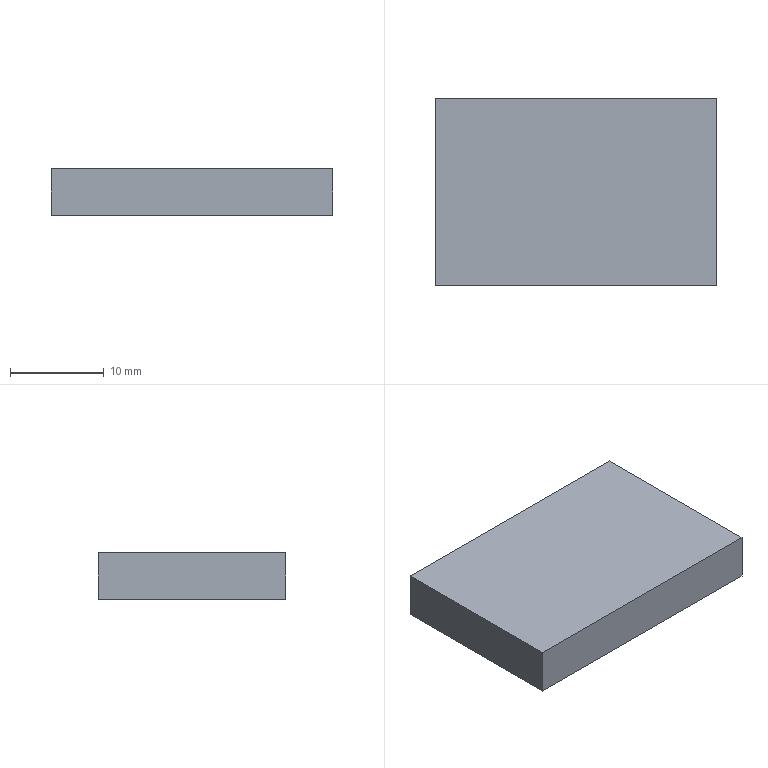Part | STEP file | MISUMI magnet MGLF5-30-20 | 1 solid | 6 faces | box 30 x 20 x 5 mm | volume 3000 mm3 | plane 6
STEP:
#1=CARTESIAN_POINT('',(0.,0.,0.));
#2=DIRECTION('',(0.,0.,1.));
#3=DIRECTION('',(1.,0.,0.));
#4=AXIS2_PLACEMENT_3D('',#1,#2,#3);
#5=CARTESIAN_POINT('',(15.,-10.,5.));
#6=VERTEX_POINT('',#5);
#7=CARTESIAN_POINT('',(15.,10.,5.));
#8=VERTEX_POINT('',#7);
#9=CARTESIAN_POINT('',(15.,0.,5.));
#10=DIRECTION('',(0.,1.,0.));
#11=VECTOR('',#10,1.);
#12=LINE('',#9,#11);
#13=CARTESIAN_POINT('',(0.,0.,5.));
#14=DIRECTION('',(0.,0.,1.));
#15=DIRECTION('',(1.,0.,0.));
#16=AXIS2_PLACEMENT_3D('',#13,#14,#15);
#17=PLANE('',#16);
#18=CARTESIAN_POINT('',(15.,0.));
#19=DIRECTION('',(0.,1.));
#20=VECTOR('',#19,1.);
#21=LINE('',#18,#20);
#22=(GEOMETRIC_REPRESENTATION_CONTEXT(2)PARAMETRIC_REPRESENTATION_CONTEXT()REPRESENTATION_CONTEXT('',''));
#23=DEFINITIONAL_REPRESENTATION('',(#21),#22);
#24=PCURVE('',#17,#23);
#25=CARTESIAN_POINT('',(15.,10.,0.));
#26=DIRECTION('',(1.,0.,0.));
#27=DIRECTION('',(0.,0.,-1.));
#28=AXIS2_PLACEMENT_3D('',#25,#26,#27);
#29=PLANE('',#28);
#30=CARTESIAN_POINT('',(-5.,-10.));
#31=DIRECTION('',(0.,1.));
#32=VECTOR('',#31,1.);
#33=LINE('',#30,#32);
#34=(GEOMETRIC_REPRESENTATION_CONTEXT(2)PARAMETRIC_REPRESENTATION_CONTEXT()REPRESENTATION_CONTEXT('',''));
#35=DEFINITIONAL_REPRESENTATION('',(#33),#34);
#36=PCURVE('',#29,#35);
#37=SURFACE_CURVE('',#12,(#24,#36),.PCURVE_S1.);
#38=EDGE_CURVE('',#6,#8,#37,.T.);
#39=ORIENTED_EDGE('',*,*,#38,.T.);
#40=CARTESIAN_POINT('',(-15.,10.,5.));
#41=VERTEX_POINT('',#40);
#42=CARTESIAN_POINT('',(0.,10.,5.));
#43=DIRECTION('',(-1.,0.,0.));
#44=VECTOR('',#43,1.);
#45=LINE('',#42,#44);
#46=CARTESIAN_POINT('',(0.,10.));
#47=DIRECTION('',(-1.,0.));
#48=VECTOR('',#47,1.);
#49=LINE('',#46,#48);
#50=(GEOMETRIC_REPRESENTATION_CONTEXT(2)PARAMETRIC_REPRESENTATION_CONTEXT()REPRESENTATION_CONTEXT('',''));
#51=DEFINITIONAL_REPRESENTATION('',(#49),#50);
#52=PCURVE('',#17,#51);
#53=CARTESIAN_POINT('',(-15.,10.,0.));
#54=DIRECTION('',(0.,1.,0.));
#55=DIRECTION('',(0.,0.,1.));
#56=AXIS2_PLACEMENT_3D('',#53,#54,#55);
#57=PLANE('',#56);
#58=CARTESIAN_POINT('',(5.,15.));
#59=DIRECTION('',(0.,-1.));
#60=VECTOR('',#59,1.);
#61=LINE('',#58,#60);
#62=(GEOMETRIC_REPRESENTATION_CONTEXT(2)PARAMETRIC_REPRESENTATION_CONTEXT()REPRESENTATION_CONTEXT('',''));
#63=DEFINITIONAL_REPRESENTATION('',(#61),#62);
#64=PCURVE('',#57,#63);
#65=SURFACE_CURVE('',#45,(#52,#64),.PCURVE_S1.);
#66=EDGE_CURVE('',#8,#41,#65,.T.);
#67=ORIENTED_EDGE('',*,*,#66,.T.);
#68=CARTESIAN_POINT('',(-15.,-10.,5.));
#69=VERTEX_POINT('',#68);
#70=CARTESIAN_POINT('',(-15.,0.,5.));
#71=DIRECTION('',(0.,-1.,0.));
#72=VECTOR('',#71,1.);
#73=LINE('',#70,#72);
#74=CARTESIAN_POINT('',(-15.,0.));
#75=DIRECTION('',(0.,-1.));
#76=VECTOR('',#75,1.);
#77=LINE('',#74,#76);
#78=(GEOMETRIC_REPRESENTATION_CONTEXT(2)PARAMETRIC_REPRESENTATION_CONTEXT()REPRESENTATION_CONTEXT('',''));
#79=DEFINITIONAL_REPRESENTATION('',(#77),#78);
#80=PCURVE('',#17,#79);
#81=CARTESIAN_POINT('',(-15.,-10.,0.));
#82=DIRECTION('',(-1.,0.,0.));
#83=DIRECTION('',(0.,0.,1.));
#84=AXIS2_PLACEMENT_3D('',#81,#82,#83);
#85=PLANE('',#84);
#86=CARTESIAN_POINT('',(5.,10.));
#87=DIRECTION('',(0.,-1.));
#88=VECTOR('',#87,1.);
#89=LINE('',#86,#88);
#90=(GEOMETRIC_REPRESENTATION_CONTEXT(2)PARAMETRIC_REPRESENTATION_CONTEXT()REPRESENTATION_CONTEXT('',''));
#91=DEFINITIONAL_REPRESENTATION('',(#89),#90);
#92=PCURVE('',#85,#91);
#93=SURFACE_CURVE('',#73,(#80,#92),.PCURVE_S1.);
#94=EDGE_CURVE('',#41,#69,#93,.T.);
#95=ORIENTED_EDGE('',*,*,#94,.T.);
#96=CARTESIAN_POINT('',(0.,-10.,5.));
#97=DIRECTION('',(1.,0.,0.));
#98=VECTOR('',#97,1.);
#99=LINE('',#96,#98);
#100=CARTESIAN_POINT('',(0.,-10.));
#101=DIRECTION('',(1.,0.));
#102=VECTOR('',#101,1.);
#103=LINE('',#100,#102);
#104=(GEOMETRIC_REPRESENTATION_CONTEXT(2)PARAMETRIC_REPRESENTATION_CONTEXT()REPRESENTATION_CONTEXT('',''));
#105=DEFINITIONAL_REPRESENTATION('',(#103),#104);
#106=PCURVE('',#17,#105);
#107=CARTESIAN_POINT('',(15.,-10.,0.));
#108=DIRECTION('',(0.,-1.,0.));
#109=DIRECTION('',(0.,0.,-1.));
#110=AXIS2_PLACEMENT_3D('',#107,#108,#109);
#111=PLANE('',#110);
#112=CARTESIAN_POINT('',(-5.,-15.));
#113=DIRECTION('',(0.,1.));
#114=VECTOR('',#113,1.);
#115=LINE('',#112,#114);
#116=(GEOMETRIC_REPRESENTATION_CONTEXT(2)PARAMETRIC_REPRESENTATION_CONTEXT()REPRESENTATION_CONTEXT('',''));
#117=DEFINITIONAL_REPRESENTATION('',(#115),#116);
#118=PCURVE('',#111,#117);
#119=SURFACE_CURVE('',#99,(#106,#118),.PCURVE_S1.);
#120=EDGE_CURVE('',#69,#6,#119,.T.);
#121=ORIENTED_EDGE('',*,*,#120,.T.);
#122=EDGE_LOOP('',(#39,#67,#95,#121));
#123=FACE_BOUND('',#122,.T.);
#124=ADVANCED_FACE('',(#123),#17,.T.);
#125=CARTESIAN_POINT('',(15.,10.,0.));
#126=VERTEX_POINT('',#125);
#127=CARTESIAN_POINT('',(-15.,10.,0.));
#128=VERTEX_POINT('',#127);
#129=CARTESIAN_POINT('',(-15.,10.,0.));
#130=DIRECTION('',(-1.,0.,0.));
#131=VECTOR('',#130,1.);
#132=LINE('',#129,#131);
#133=CARTESIAN_POINT('',(0.,0.));
#134=DIRECTION('',(0.,-1.));
#135=VECTOR('',#134,1.);
#136=LINE('',#133,#135);
#137=(GEOMETRIC_REPRESENTATION_CONTEXT(2)PARAMETRIC_REPRESENTATION_CONTEXT()REPRESENTATION_CONTEXT('',''));
#138=DEFINITIONAL_REPRESENTATION('',(#136),#137);
#139=PCURVE('',#57,#138);
#140=CARTESIAN_POINT('',(0.,0.,0.));
#141=DIRECTION('',(0.,0.,1.));
#142=DIRECTION('',(1.,0.,0.));
#143=AXIS2_PLACEMENT_3D('',#140,#141,#142);
#144=PLANE('',#143);
#145=CARTESIAN_POINT('',(-15.,10.));
#146=DIRECTION('',(-1.,0.));
#147=VECTOR('',#146,1.);
#148=LINE('',#145,#147);
#149=(GEOMETRIC_REPRESENTATION_CONTEXT(2)PARAMETRIC_REPRESENTATION_CONTEXT()REPRESENTATION_CONTEXT('',''));
#150=DEFINITIONAL_REPRESENTATION('',(#148),#149);
#151=PCURVE('',#144,#150);
#152=SURFACE_CURVE('',#132,(#139,#151),.PCURVE_S1.);
#153=EDGE_CURVE('',#126,#128,#152,.T.);
#154=ORIENTED_EDGE('',*,*,#153,.T.);
#155=CARTESIAN_POINT('',(-15.,10.,0.));
#156=DIRECTION('',(0.,0.,1.));
#157=VECTOR('',#156,1.);
#158=LINE('',#155,#157);
#159=CARTESIAN_POINT('',(0.,0.));
#160=DIRECTION('',(1.,0.));
#161=VECTOR('',#160,1.);
#162=LINE('',#159,#161);
#163=(GEOMETRIC_REPRESENTATION_CONTEXT(2)PARAMETRIC_REPRESENTATION_CONTEXT()REPRESENTATION_CONTEXT('',''));
#164=DEFINITIONAL_REPRESENTATION('',(#162),#163);
#165=PCURVE('',#57,#164);
#166=CARTESIAN_POINT('',(0.,20.));
#167=DIRECTION('',(1.,0.));
#168=VECTOR('',#167,1.);
#169=LINE('',#166,#168);
#170=(GEOMETRIC_REPRESENTATION_CONTEXT(2)PARAMETRIC_REPRESENTATION_CONTEXT()REPRESENTATION_CONTEXT('',''));
#171=DEFINITIONAL_REPRESENTATION('',(#169),#170);
#172=PCURVE('',#85,#171);
#173=SURFACE_CURVE('',#158,(#165,#172),.PCURVE_S1.);
#174=EDGE_CURVE('',#128,#41,#173,.T.);
#175=ORIENTED_EDGE('',*,*,#174,.T.);
#176=ORIENTED_EDGE('',*,*,#66,.F.);
#177=CARTESIAN_POINT('',(15.,10.,0.));
#178=DIRECTION('',(0.,0.,-1.));
#179=VECTOR('',#178,1.);
#180=LINE('',#177,#179);
#181=CARTESIAN_POINT('',(0.,30.));
#182=DIRECTION('',(-1.,0.));
#183=VECTOR('',#182,1.);
#184=LINE('',#181,#183);
#185=(GEOMETRIC_REPRESENTATION_CONTEXT(2)PARAMETRIC_REPRESENTATION_CONTEXT()REPRESENTATION_CONTEXT('',''));
#186=DEFINITIONAL_REPRESENTATION('',(#184),#185);
#187=PCURVE('',#57,#186);
#188=CARTESIAN_POINT('',(0.,0.));
#189=DIRECTION('',(1.,0.));
#190=VECTOR('',#189,1.);
#191=LINE('',#188,#190);
#192=(GEOMETRIC_REPRESENTATION_CONTEXT(2)PARAMETRIC_REPRESENTATION_CONTEXT()REPRESENTATION_CONTEXT('',''));
#193=DEFINITIONAL_REPRESENTATION('',(#191),#192);
#194=PCURVE('',#29,#193);
#195=SURFACE_CURVE('',#180,(#187,#194),.PCURVE_S1.);
#196=EDGE_CURVE('',#8,#126,#195,.T.);
#197=ORIENTED_EDGE('',*,*,#196,.T.);
#198=EDGE_LOOP('',(#154,#175,#176,#197));
#199=FACE_BOUND('',#198,.T.);
#200=ADVANCED_FACE('',(#199),#57,.T.);
#201=CARTESIAN_POINT('',(15.,-10.,0.));
#202=VERTEX_POINT('',#201);
#203=CARTESIAN_POINT('',(15.,10.,0.));
#204=DIRECTION('',(0.,1.,0.));
#205=VECTOR('',#204,1.);
#206=LINE('',#203,#205);
#207=CARTESIAN_POINT('',(0.,0.));
#208=DIRECTION('',(0.,1.));
#209=VECTOR('',#208,1.);
#210=LINE('',#207,#209);
#211=(GEOMETRIC_REPRESENTATION_CONTEXT(2)PARAMETRIC_REPRESENTATION_CONTEXT()REPRESENTATION_CONTEXT('',''));
#212=DEFINITIONAL_REPRESENTATION('',(#210),#211);
#213=PCURVE('',#29,#212);
#214=CARTESIAN_POINT('',(15.,10.));
#215=DIRECTION('',(0.,1.));
#216=VECTOR('',#215,1.);
#217=LINE('',#214,#216);
#218=(GEOMETRIC_REPRESENTATION_CONTEXT(2)PARAMETRIC_REPRESENTATION_CONTEXT()REPRESENTATION_CONTEXT('',''));
#219=DEFINITIONAL_REPRESENTATION('',(#217),#218);
#220=PCURVE('',#144,#219);
#221=SURFACE_CURVE('',#206,(#213,#220),.PCURVE_S1.);
#222=EDGE_CURVE('',#202,#126,#221,.T.);
#223=ORIENTED_EDGE('',*,*,#222,.T.);
#224=ORIENTED_EDGE('',*,*,#196,.F.);
#225=ORIENTED_EDGE('',*,*,#38,.F.);
#226=CARTESIAN_POINT('',(15.,-10.,0.));
#227=DIRECTION('',(0.,0.,-1.));
#228=VECTOR('',#227,1.);
#229=LINE('',#226,#228);
#230=CARTESIAN_POINT('',(0.,-20.));
#231=DIRECTION('',(1.,0.));
#232=VECTOR('',#231,1.);
#233=LINE('',#230,#232);
#234=(GEOMETRIC_REPRESENTATION_CONTEXT(2)PARAMETRIC_REPRESENTATION_CONTEXT()REPRESENTATION_CONTEXT('',''));
#235=DEFINITIONAL_REPRESENTATION('',(#233),#234);
#236=PCURVE('',#29,#235);
#237=CARTESIAN_POINT('',(0.,0.));
#238=DIRECTION('',(1.,0.));
#239=VECTOR('',#238,1.);
#240=LINE('',#237,#239);
#241=(GEOMETRIC_REPRESENTATION_CONTEXT(2)PARAMETRIC_REPRESENTATION_CONTEXT()REPRESENTATION_CONTEXT('',''));
#242=DEFINITIONAL_REPRESENTATION('',(#240),#241);
#243=PCURVE('',#111,#242);
#244=SURFACE_CURVE('',#229,(#236,#243),.PCURVE_S1.);
#245=EDGE_CURVE('',#6,#202,#244,.T.);
#246=ORIENTED_EDGE('',*,*,#245,.T.);
#247=EDGE_LOOP('',(#223,#224,#225,#246));
#248=FACE_BOUND('',#247,.T.);
#249=ADVANCED_FACE('',(#248),#29,.T.);
#250=CARTESIAN_POINT('',(-15.,-10.,0.));
#251=VERTEX_POINT('',#250);
#252=CARTESIAN_POINT('',(15.,-10.,0.));
#253=DIRECTION('',(1.,0.,0.));
#254=VECTOR('',#253,1.);
#255=LINE('',#252,#254);
#256=CARTESIAN_POINT('',(0.,0.));
#257=DIRECTION('',(0.,1.));
#258=VECTOR('',#257,1.);
#259=LINE('',#256,#258);
#260=(GEOMETRIC_REPRESENTATION_CONTEXT(2)PARAMETRIC_REPRESENTATION_CONTEXT()REPRESENTATION_CONTEXT('',''));
#261=DEFINITIONAL_REPRESENTATION('',(#259),#260);
#262=PCURVE('',#111,#261);
#263=CARTESIAN_POINT('',(15.,-10.));
#264=DIRECTION('',(1.,0.));
#265=VECTOR('',#264,1.);
#266=LINE('',#263,#265);
#267=(GEOMETRIC_REPRESENTATION_CONTEXT(2)PARAMETRIC_REPRESENTATION_CONTEXT()REPRESENTATION_CONTEXT('',''));
#268=DEFINITIONAL_REPRESENTATION('',(#266),#267);
#269=PCURVE('',#144,#268);
#270=SURFACE_CURVE('',#255,(#262,#269),.PCURVE_S1.);
#271=EDGE_CURVE('',#251,#202,#270,.T.);
#272=ORIENTED_EDGE('',*,*,#271,.T.);
#273=ORIENTED_EDGE('',*,*,#245,.F.);
#274=ORIENTED_EDGE('',*,*,#120,.F.);
#275=CARTESIAN_POINT('',(-15.,-10.,0.));
#276=DIRECTION('',(0.,0.,-1.));
#277=VECTOR('',#276,1.);
#278=LINE('',#275,#277);
#279=CARTESIAN_POINT('',(0.,-30.));
#280=DIRECTION('',(1.,0.));
#281=VECTOR('',#280,1.);
#282=LINE('',#279,#281);
#283=(GEOMETRIC_REPRESENTATION_CONTEXT(2)PARAMETRIC_REPRESENTATION_CONTEXT()REPRESENTATION_CONTEXT('',''));
#284=DEFINITIONAL_REPRESENTATION('',(#282),#283);
#285=PCURVE('',#111,#284);
#286=CARTESIAN_POINT('',(0.,0.));
#287=DIRECTION('',(-1.,0.));
#288=VECTOR('',#287,1.);
#289=LINE('',#286,#288);
#290=(GEOMETRIC_REPRESENTATION_CONTEXT(2)PARAMETRIC_REPRESENTATION_CONTEXT()REPRESENTATION_CONTEXT('',''));
#291=DEFINITIONAL_REPRESENTATION('',(#289),#290);
#292=PCURVE('',#85,#291);
#293=SURFACE_CURVE('',#278,(#285,#292),.PCURVE_S1.);
#294=EDGE_CURVE('',#69,#251,#293,.T.);
#295=ORIENTED_EDGE('',*,*,#294,.T.);
#296=EDGE_LOOP('',(#272,#273,#274,#295));
#297=FACE_BOUND('',#296,.T.);
#298=ADVANCED_FACE('',(#297),#111,.T.);
#299=CARTESIAN_POINT('',(-15.,-10.,0.));
#300=DIRECTION('',(0.,-1.,0.));
#301=VECTOR('',#300,1.);
#302=LINE('',#299,#301);
#303=CARTESIAN_POINT('',(0.,0.));
#304=DIRECTION('',(0.,-1.));
#305=VECTOR('',#304,1.);
#306=LINE('',#303,#305);
#307=(GEOMETRIC_REPRESENTATION_CONTEXT(2)PARAMETRIC_REPRESENTATION_CONTEXT()REPRESENTATION_CONTEXT('',''));
#308=DEFINITIONAL_REPRESENTATION('',(#306),#307);
#309=PCURVE('',#85,#308);
#310=CARTESIAN_POINT('',(-15.,-10.));
#311=DIRECTION('',(0.,-1.));
#312=VECTOR('',#311,1.);
#313=LINE('',#310,#312);
#314=(GEOMETRIC_REPRESENTATION_CONTEXT(2)PARAMETRIC_REPRESENTATION_CONTEXT()REPRESENTATION_CONTEXT('',''));
#315=DEFINITIONAL_REPRESENTATION('',(#313),#314);
#316=PCURVE('',#144,#315);
#317=SURFACE_CURVE('',#302,(#309,#316),.PCURVE_S1.);
#318=EDGE_CURVE('',#128,#251,#317,.T.);
#319=ORIENTED_EDGE('',*,*,#318,.T.);
#320=ORIENTED_EDGE('',*,*,#294,.F.);
#321=ORIENTED_EDGE('',*,*,#94,.F.);
#322=ORIENTED_EDGE('',*,*,#174,.F.);
#323=EDGE_LOOP('',(#319,#320,#321,#322));
#324=FACE_BOUND('',#323,.T.);
#325=ADVANCED_FACE('',(#324),#85,.T.);
#326=ORIENTED_EDGE('',*,*,#318,.F.);
#327=ORIENTED_EDGE('',*,*,#153,.F.);
#328=ORIENTED_EDGE('',*,*,#222,.F.);
#329=ORIENTED_EDGE('',*,*,#271,.F.);
#330=EDGE_LOOP('',(#326,#327,#328,#329));
#331=FACE_BOUND('',#330,.T.);
#332=ADVANCED_FACE('',(#331),#144,.F.);
#333=CLOSED_SHELL('',(#124,#200,#249,#298,#325,#332));
#334=MANIFOLD_SOLID_BREP('',#333);
#335=(LENGTH_UNIT()NAMED_UNIT(*)SI_UNIT(.MILLI.,.METRE.));
#336=UNCERTAINTY_MEASURE_WITH_UNIT(LENGTH_MEASURE(0.0000001),#335,'','');
#337=(NAMED_UNIT(*)PLANE_ANGLE_UNIT()SI_UNIT($,.RADIAN.));
#338=(NAMED_UNIT(*)SI_UNIT($,.STERADIAN.)SOLID_ANGLE_UNIT());
#339=(GEOMETRIC_REPRESENTATION_CONTEXT(3)GLOBAL_UNCERTAINTY_ASSIGNED_CONTEXT((#336))GLOBAL_UNIT_ASSIGNED_CONTEXT((#335,#337,#338))REPRESENTATION_CONTEXT('',''));
#340=ADVANCED_BREP_SHAPE_REPRESENTATION('',(#4,#334),#339);